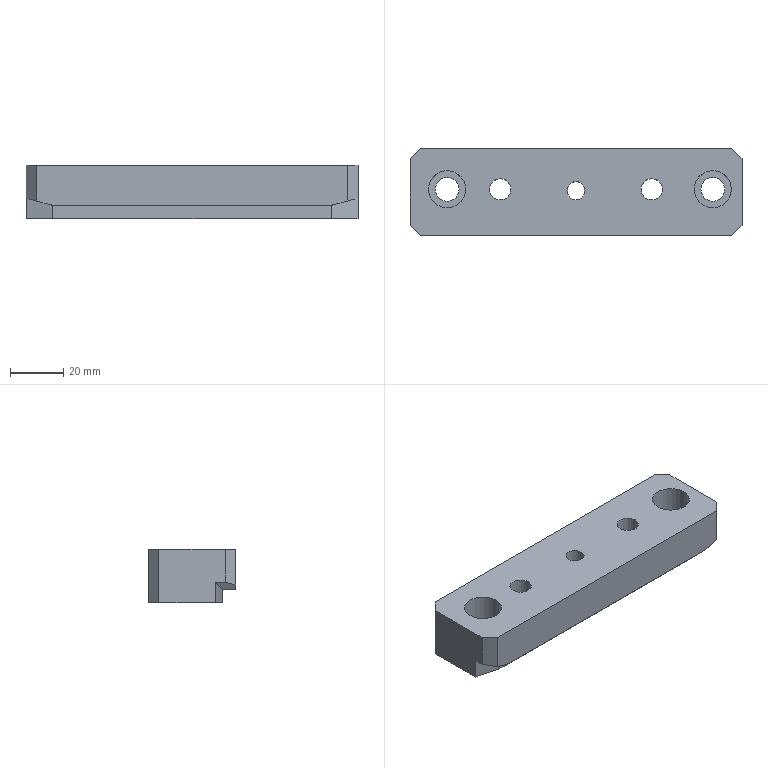Part | NX | features 20 2 | 1 solid | 25 faces | box 125 x 33 x 20 mm | volume 71448 mm3 | plane 18 | cylinder 7 | commonest cylinder face diameters 8.001 x2 9 x2 14 x2 6.8 x1
STEP:
#1=CARTESIAN_POINT('',(3433.002,435.,-3.5));
#2=VERTEX_POINT('',#1);
#3=CARTESIAN_POINT('',(3428.502,435.,-3.5));
#4=DIRECTION('',(0.,0.,-1.));
#5=DIRECTION('',(1.,0.,0.));
#6=AXIS2_PLACEMENT_3D('',#3,#4,#5);
#7=CIRCLE('',#6,4.5);
#8=EDGE_CURVE('',#2,#2,#7,.T.);
#9=ORIENTED_EDGE('',*,*,#8,.F.);
#10=EDGE_LOOP('',(#9));
#11=FACE_BOUND('',#10,.T.);
#12=CARTESIAN_POINT('',(3380.402,434.5,-3.5));
#13=VERTEX_POINT('',#12);
#14=CARTESIAN_POINT('',(3377.002,434.5,-3.5));
#15=DIRECTION('',(0.,0.,-1.));
#16=DIRECTION('',(1.,0.,0.));
#17=AXIS2_PLACEMENT_3D('',#14,#15,#16);
#18=CIRCLE('',#17,3.4);
#19=EDGE_CURVE('',#13,#13,#18,.T.);
#20=ORIENTED_EDGE('',*,*,#19,.F.);
#21=EDGE_LOOP('',(#20));
#22=FACE_BOUND('',#21,.T.);
#23=CARTESIAN_POINT('',(3333.002,435.,-3.5));
#24=VERTEX_POINT('',#23);
#25=CARTESIAN_POINT('',(3328.502,435.,-3.5));
#26=DIRECTION('',(0.,0.,1.));
#27=DIRECTION('',(1.,0.,0.));
#28=AXIS2_PLACEMENT_3D('',#25,#26,#27);
#29=CIRCLE('',#28,4.5);
#30=EDGE_CURVE('',#24,#24,#29,.T.);
#31=ORIENTED_EDGE('',*,*,#30,.T.);
#32=EDGE_LOOP('',(#31));
#33=FACE_BOUND('',#32,.T.);
#34=CARTESIAN_POINT('',(3429.501,422.5,-3.5));
#35=VERTEX_POINT('',#34);
#36=CARTESIAN_POINT('',(3324.501,422.5,-3.5));
#37=VERTEX_POINT('',#36);
#38=CARTESIAN_POINT('',(3410.501,422.5,-3.5));
#39=DIRECTION('',(-1.,0.,0.));
#40=VECTOR('',#39,1000.);
#41=LINE('',#38,#40);
#42=EDGE_CURVE('',#35,#37,#41,.T.);
#43=ORIENTED_EDGE('',*,*,#42,.T.);
#44=CARTESIAN_POINT('',(3314.502,425.179,-3.5));
#45=VERTEX_POINT('',#44);
#46=CARTESIAN_POINT('',(3324.501,422.5,-3.5));
#47=DIRECTION('',(-0.9659,0.2588,0.));
#48=VECTOR('',#47,1000.);
#49=LINE('',#46,#48);
#50=EDGE_CURVE('',#37,#45,#49,.T.);
#51=ORIENTED_EDGE('',*,*,#50,.T.);
#52=CARTESIAN_POINT('',(3314.502,446.5,-3.5));
#53=VERTEX_POINT('',#52);
#54=CARTESIAN_POINT('',(3314.502,417.5,-3.5));
#55=DIRECTION('',(0.,1.,0.));
#56=VECTOR('',#55,1000.);
#57=LINE('',#54,#56);
#58=EDGE_CURVE('',#45,#53,#57,.T.);
#59=ORIENTED_EDGE('',*,*,#58,.T.);
#60=CARTESIAN_POINT('',(3318.502,450.5,-3.5));
#61=VERTEX_POINT('',#60);
#62=CARTESIAN_POINT('',(3318.502,450.5,-3.5));
#63=DIRECTION('',(-0.7071,-0.7071,0.));
#64=VECTOR('',#63,1000.);
#65=LINE('',#62,#64);
#66=EDGE_CURVE('',#61,#53,#65,.T.);
#67=ORIENTED_EDGE('',*,*,#66,.F.);
#68=CARTESIAN_POINT('',(3435.502,450.5,-3.5));
#69=VERTEX_POINT('',#68);
#70=CARTESIAN_POINT('',(3432.502,450.5,-3.5));
#71=DIRECTION('',(1.,0.,0.));
#72=VECTOR('',#71,1000.);
#73=LINE('',#70,#72);
#74=EDGE_CURVE('',#61,#69,#73,.T.);
#75=ORIENTED_EDGE('',*,*,#74,.T.);
#76=CARTESIAN_POINT('',(3439.502,446.5,-3.5));
#77=VERTEX_POINT('',#76);
#78=CARTESIAN_POINT('',(3439.502,446.5,-3.5));
#79=DIRECTION('',(-0.7071,0.7071,0.));
#80=VECTOR('',#79,1000.);
#81=LINE('',#78,#80);
#82=EDGE_CURVE('',#77,#69,#81,.T.);
#83=ORIENTED_EDGE('',*,*,#82,.F.);
#84=CARTESIAN_POINT('',(3439.502,425.18,-3.5));
#85=VERTEX_POINT('',#84);
#86=CARTESIAN_POINT('',(3439.502,450.5,-3.5));
#87=DIRECTION('',(0.,-1.,0.));
#88=VECTOR('',#87,1000.);
#89=LINE('',#86,#88);
#90=EDGE_CURVE('',#77,#85,#89,.T.);
#91=ORIENTED_EDGE('',*,*,#90,.T.);
#92=CARTESIAN_POINT('',(3439.502,425.18,-3.5));
#93=DIRECTION('',(-0.9659,-0.2588,0.));
#94=VECTOR('',#93,1000.);
#95=LINE('',#92,#94);
#96=EDGE_CURVE('',#85,#35,#95,.T.);
#97=ORIENTED_EDGE('',*,*,#96,.T.);
#98=EDGE_LOOP('',(#43,#51,#59,#67,#75,#83,#91,#97));
#99=FACE_BOUND('',#98,.T.);
#100=CARTESIAN_POINT('',(3352.503,435.,-3.5));
#101=VERTEX_POINT('',#100);
#102=CARTESIAN_POINT('',(3348.502,435.,-3.5));
#103=DIRECTION('',(0.,0.,1.));
#104=DIRECTION('',(1.,0.,0.));
#105=AXIS2_PLACEMENT_3D('',#102,#103,#104);
#106=CIRCLE('',#105,4.);
#107=EDGE_CURVE('',#101,#101,#106,.T.);
#108=ORIENTED_EDGE('',*,*,#107,.T.);
#109=EDGE_LOOP('',(#108));
#110=FACE_BOUND('',#109,.T.);
#111=CARTESIAN_POINT('',(3409.503,435.,-3.5));
#112=VERTEX_POINT('',#111);
#113=CARTESIAN_POINT('',(3405.502,435.,-3.5));
#114=DIRECTION('',(0.,0.,-1.));
#115=DIRECTION('',(1.,0.,0.));
#116=AXIS2_PLACEMENT_3D('',#113,#114,#115);
#117=CIRCLE('',#116,4.);
#118=EDGE_CURVE('',#112,#112,#117,.T.);
#119=ORIENTED_EDGE('',*,*,#118,.F.);
#120=EDGE_LOOP('',(#119));
#121=FACE_BOUND('',#120,.T.);
#122=CARTESIAN_POINT('',(3502.502,450.5,-3.5));
#123=DIRECTION('',(0.,0.,1.));
#124=DIRECTION('',(-1.,0.,0.));
#125=AXIS2_PLACEMENT_3D('',#122,#123,#124);
#126=PLANE('',#125);
#127=ADVANCED_FACE('',(#11,#22,#33,#99,#110,#121),#126,.F.);
#128=CARTESIAN_POINT('',(3324.502,417.5,1.5));
#129=VERTEX_POINT('',#128);
#130=CARTESIAN_POINT('',(3429.502,417.5,1.5));
#131=VERTEX_POINT('',#130);
#132=CARTESIAN_POINT('',(3450.502,417.5,1.5));
#133=DIRECTION('',(1.,0.,0.));
#134=VECTOR('',#133,1000.);
#135=LINE('',#132,#134);
#136=EDGE_CURVE('',#129,#131,#135,.T.);
#137=ORIENTED_EDGE('',*,*,#136,.T.);
#138=CARTESIAN_POINT('',(3435.502,417.5,3.108));
#139=VERTEX_POINT('',#138);
#140=CARTESIAN_POINT('',(3429.502,417.5,1.5));
#141=DIRECTION('',(-0.9659,0.,-0.2588));
#142=VECTOR('',#141,1000.);
#143=LINE('',#140,#142);
#144=EDGE_CURVE('',#139,#131,#143,.T.);
#145=ORIENTED_EDGE('',*,*,#144,.F.);
#146=CARTESIAN_POINT('',(3435.502,417.5,16.5));
#147=VERTEX_POINT('',#146);
#148=CARTESIAN_POINT('',(3435.502,417.5,11.5));
#149=DIRECTION('',(0.,0.,-1.));
#150=VECTOR('',#149,1000.);
#151=LINE('',#148,#150);
#152=EDGE_CURVE('',#147,#139,#151,.T.);
#153=ORIENTED_EDGE('',*,*,#152,.F.);
#154=CARTESIAN_POINT('',(3318.502,417.5,16.5));
#155=VERTEX_POINT('',#154);
#156=CARTESIAN_POINT('',(3472.502,417.5,16.5));
#157=DIRECTION('',(-1.,0.,0.));
#158=VECTOR('',#157,1000.);
#159=LINE('',#156,#158);
#160=EDGE_CURVE('',#147,#155,#159,.T.);
#161=ORIENTED_EDGE('',*,*,#160,.T.);
#162=CARTESIAN_POINT('',(3318.502,417.5,3.108));
#163=VERTEX_POINT('',#162);
#164=CARTESIAN_POINT('',(3318.502,417.5,11.5));
#165=DIRECTION('',(0.,0.,1.));
#166=VECTOR('',#165,1000.);
#167=LINE('',#164,#166);
#168=EDGE_CURVE('',#163,#155,#167,.T.);
#169=ORIENTED_EDGE('',*,*,#168,.F.);
#170=CARTESIAN_POINT('',(3324.502,417.5,1.5));
#171=DIRECTION('',(-0.9659,0.,0.2588));
#172=VECTOR('',#171,1000.);
#173=LINE('',#170,#172);
#174=EDGE_CURVE('',#129,#163,#173,.T.);
#175=ORIENTED_EDGE('',*,*,#174,.F.);
#176=EDGE_LOOP('',(#137,#145,#153,#161,#169,#175));
#177=FACE_BOUND('',#176,.T.);
#178=CARTESIAN_POINT('',(3472.502,417.5,11.5));
#179=DIRECTION('',(0.,1.,0.));
#180=DIRECTION('',(0.,0.,1.));
#181=AXIS2_PLACEMENT_3D('',#178,#179,#180);
#182=PLANE('',#181);
#183=ADVANCED_FACE('',(#177),#182,.F.);
#184=CARTESIAN_POINT('',(3409.503,435.,16.5));
#185=VERTEX_POINT('',#184);
#186=CARTESIAN_POINT('',(3405.502,435.,16.5));
#187=DIRECTION('',(0.,0.,1.));
#188=DIRECTION('',(1.,0.,0.));
#189=AXIS2_PLACEMENT_3D('',#186,#187,#188);
#190=CIRCLE('',#189,4.);
#191=EDGE_CURVE('',#185,#185,#190,.T.);
#192=ORIENTED_EDGE('',*,*,#191,.F.);
#193=EDGE_LOOP('',(#192));
#194=FACE_BOUND('',#193,.T.);
#195=CARTESIAN_POINT('',(3352.503,435.,16.5));
#196=VERTEX_POINT('',#195);
#197=CARTESIAN_POINT('',(3348.502,435.,16.5));
#198=DIRECTION('',(0.,0.,1.));
#199=DIRECTION('',(1.,0.,0.));
#200=AXIS2_PLACEMENT_3D('',#197,#198,#199);
#201=CIRCLE('',#200,4.);
#202=EDGE_CURVE('',#196,#196,#201,.T.);
#203=ORIENTED_EDGE('',*,*,#202,.F.);
#204=EDGE_LOOP('',(#203));
#205=FACE_BOUND('',#204,.T.);
#206=CARTESIAN_POINT('',(3435.502,435.,16.5));
#207=VERTEX_POINT('',#206);
#208=CARTESIAN_POINT('',(3428.502,435.,16.5));
#209=DIRECTION('',(0.,0.,-1.));
#210=DIRECTION('',(1.,0.,0.));
#211=AXIS2_PLACEMENT_3D('',#208,#209,#210);
#212=CIRCLE('',#211,7.);
#213=EDGE_CURVE('',#207,#207,#212,.T.);
#214=ORIENTED_EDGE('',*,*,#213,.T.);
#215=EDGE_LOOP('',(#214));
#216=FACE_BOUND('',#215,.T.);
#217=CARTESIAN_POINT('',(3335.502,435.,16.5));
#218=VERTEX_POINT('',#217);
#219=CARTESIAN_POINT('',(3328.502,435.,16.5));
#220=DIRECTION('',(0.,0.,-1.));
#221=DIRECTION('',(1.,0.,0.));
#222=AXIS2_PLACEMENT_3D('',#219,#220,#221);
#223=CIRCLE('',#222,7.);
#224=EDGE_CURVE('',#218,#218,#223,.T.);
#225=ORIENTED_EDGE('',*,*,#224,.T.);
#226=EDGE_LOOP('',(#225));
#227=FACE_BOUND('',#226,.T.);
#228=ORIENTED_EDGE('',*,*,#160,.F.);
#229=CARTESIAN_POINT('',(3439.502,421.5,16.5));
#230=VERTEX_POINT('',#229);
#231=CARTESIAN_POINT('',(3435.502,417.5,16.5));
#232=DIRECTION('',(-0.7071,-0.7071,0.));
#233=VECTOR('',#232,1000.);
#234=LINE('',#231,#233);
#235=EDGE_CURVE('',#230,#147,#234,.T.);
#236=ORIENTED_EDGE('',*,*,#235,.F.);
#237=CARTESIAN_POINT('',(3439.502,446.5,16.5));
#238=VERTEX_POINT('',#237);
#239=CARTESIAN_POINT('',(3439.502,450.5,16.5));
#240=DIRECTION('',(0.,-1.,0.));
#241=VECTOR('',#240,1000.);
#242=LINE('',#239,#241);
#243=EDGE_CURVE('',#238,#230,#242,.T.);
#244=ORIENTED_EDGE('',*,*,#243,.F.);
#245=CARTESIAN_POINT('',(3435.502,450.5,16.5));
#246=VERTEX_POINT('',#245);
#247=CARTESIAN_POINT('',(3439.502,446.5,16.5));
#248=DIRECTION('',(0.7071,-0.7071,0.));
#249=VECTOR('',#248,1000.);
#250=LINE('',#247,#249);
#251=EDGE_CURVE('',#246,#238,#250,.T.);
#252=ORIENTED_EDGE('',*,*,#251,.F.);
#253=CARTESIAN_POINT('',(3318.502,450.5,16.5));
#254=VERTEX_POINT('',#253);
#255=CARTESIAN_POINT('',(3392.502,450.5,16.5));
#256=DIRECTION('',(1.,0.,0.));
#257=VECTOR('',#256,1000.);
#258=LINE('',#255,#257);
#259=EDGE_CURVE('',#254,#246,#258,.T.);
#260=ORIENTED_EDGE('',*,*,#259,.F.);
#261=CARTESIAN_POINT('',(3314.502,446.5,16.5));
#262=VERTEX_POINT('',#261);
#263=CARTESIAN_POINT('',(3318.502,450.5,16.5));
#264=DIRECTION('',(0.7071,0.7071,0.));
#265=VECTOR('',#264,1000.);
#266=LINE('',#263,#265);
#267=EDGE_CURVE('',#262,#254,#266,.T.);
#268=ORIENTED_EDGE('',*,*,#267,.F.);
#269=CARTESIAN_POINT('',(3314.502,421.5,16.5));
#270=VERTEX_POINT('',#269);
#271=CARTESIAN_POINT('',(3314.502,417.5,16.5));
#272=DIRECTION('',(0.,1.,0.));
#273=VECTOR('',#272,1000.);
#274=LINE('',#271,#273);
#275=EDGE_CURVE('',#270,#262,#274,.T.);
#276=ORIENTED_EDGE('',*,*,#275,.F.);
#277=CARTESIAN_POINT('',(3314.502,421.5,16.5));
#278=DIRECTION('',(-0.7071,0.7071,0.));
#279=VECTOR('',#278,1000.);
#280=LINE('',#277,#279);
#281=EDGE_CURVE('',#155,#270,#280,.T.);
#282=ORIENTED_EDGE('',*,*,#281,.F.);
#283=EDGE_LOOP('',(#228,#236,#244,#252,#260,#268,#276,#282));
#284=FACE_BOUND('',#283,.T.);
#285=CARTESIAN_POINT('',(3380.402,434.5,16.5));
#286=VERTEX_POINT('',#285);
#287=CARTESIAN_POINT('',(3377.002,434.5,16.5));
#288=DIRECTION('',(0.,0.,1.));
#289=DIRECTION('',(1.,0.,0.));
#290=AXIS2_PLACEMENT_3D('',#287,#288,#289);
#291=CIRCLE('',#290,3.4);
#292=EDGE_CURVE('',#286,#286,#291,.T.);
#293=ORIENTED_EDGE('',*,*,#292,.F.);
#294=EDGE_LOOP('',(#293));
#295=FACE_BOUND('',#294,.T.);
#296=CARTESIAN_POINT('',(3472.502,450.5,16.5));
#297=DIRECTION('',(0.,0.,1.));
#298=DIRECTION('',(-1.,0.,0.));
#299=AXIS2_PLACEMENT_3D('',#296,#297,#298);
#300=PLANE('',#299);
#301=ADVANCED_FACE('',(#194,#205,#216,#227,#284,#295),#300,.T.);
#302=CARTESIAN_POINT('',(3424.002,435.,6.5));
#303=VERTEX_POINT('',#302);
#304=CARTESIAN_POINT('',(3428.502,435.,6.5));
#305=DIRECTION('',(0.,0.,1.));
#306=DIRECTION('',(-1.,0.,0.));
#307=AXIS2_PLACEMENT_3D('',#304,#305,#306);
#308=CIRCLE('',#307,4.5);
#309=EDGE_CURVE('',#303,#303,#308,.T.);
#310=ORIENTED_EDGE('',*,*,#309,.F.);
#311=EDGE_LOOP('',(#310));
#312=FACE_BOUND('',#311,.T.);
#313=CARTESIAN_POINT('',(3421.502,435.,6.5));
#314=VERTEX_POINT('',#313);
#315=CARTESIAN_POINT('',(3428.502,435.,6.5));
#316=DIRECTION('',(0.,0.,-1.));
#317=DIRECTION('',(-1.,0.,0.));
#318=AXIS2_PLACEMENT_3D('',#315,#316,#317);
#319=CIRCLE('',#318,7.);
#320=EDGE_CURVE('',#314,#314,#319,.T.);
#321=ORIENTED_EDGE('',*,*,#320,.F.);
#322=EDGE_LOOP('',(#321));
#323=FACE_BOUND('',#322,.T.);
#324=CARTESIAN_POINT('',(3428.502,432.5,6.5));
#325=DIRECTION('',(0.,0.,-1.));
#326=DIRECTION('',(1.,0.,0.));
#327=AXIS2_PLACEMENT_3D('',#324,#325,#326);
#328=PLANE('',#327);
#329=ADVANCED_FACE('',(#312,#323),#328,.F.);
#330=CARTESIAN_POINT('',(3429.502,422.5,1.5));
#331=VERTEX_POINT('',#330);
#332=CARTESIAN_POINT('',(3429.502,425.18,1.5));
#333=DIRECTION('',(0.,1.,0.));
#334=VECTOR('',#333,1000.);
#335=LINE('',#332,#334);
#336=EDGE_CURVE('',#131,#331,#335,.T.);
#337=ORIENTED_EDGE('',*,*,#336,.T.);
#338=CARTESIAN_POINT('',(3439.502,425.18,4.179));
#339=VERTEX_POINT('',#338);
#340=CARTESIAN_POINT('',(3438.875,425.012,4.011));
#341=DIRECTION('',(0.9351,0.2506,0.2506));
#342=VECTOR('',#341,1000.);
#343=LINE('',#340,#342);
#344=EDGE_CURVE('',#331,#339,#343,.T.);
#345=ORIENTED_EDGE('',*,*,#344,.T.);
#346=CARTESIAN_POINT('',(3439.502,421.5,4.179));
#347=VERTEX_POINT('',#346);
#348=CARTESIAN_POINT('',(3439.502,417.5,4.179));
#349=DIRECTION('',(0.,-1.,0.));
#350=VECTOR('',#349,1000.);
#351=LINE('',#348,#350);
#352=EDGE_CURVE('',#339,#347,#351,.T.);
#353=ORIENTED_EDGE('',*,*,#352,.T.);
#354=CARTESIAN_POINT('',(3422.451,404.449,-0.3894));
#355=DIRECTION('',(0.6947,0.6947,0.1862));
#356=VECTOR('',#355,1000.);
#357=LINE('',#354,#356);
#358=EDGE_CURVE('',#139,#347,#357,.T.);
#359=ORIENTED_EDGE('',*,*,#358,.F.);
#360=ORIENTED_EDGE('',*,*,#144,.T.);
#361=EDGE_LOOP('',(#337,#345,#353,#359,#360));
#362=FACE_BOUND('',#361,.T.);
#363=CARTESIAN_POINT('',(3429.502,396.891,1.5));
#364=DIRECTION('',(0.2588,0.,-0.9659));
#365=DIRECTION('',(0.9659,0.,0.2588));
#366=AXIS2_PLACEMENT_3D('',#363,#364,#365);
#367=PLANE('',#366);
#368=ADVANCED_FACE('',(#362),#367,.T.);
#369=CARTESIAN_POINT('',(3324.002,435.,6.5));
#370=VERTEX_POINT('',#369);
#371=CARTESIAN_POINT('',(3328.502,435.,6.5));
#372=DIRECTION('',(0.,0.,1.));
#373=DIRECTION('',(-1.,0.,0.));
#374=AXIS2_PLACEMENT_3D('',#371,#372,#373);
#375=CIRCLE('',#374,4.5);
#376=EDGE_CURVE('',#370,#370,#375,.T.);
#377=ORIENTED_EDGE('',*,*,#376,.F.);
#378=EDGE_LOOP('',(#377));
#379=FACE_BOUND('',#378,.T.);
#380=CARTESIAN_POINT('',(3321.502,435.,6.5));
#381=VERTEX_POINT('',#380);
#382=CARTESIAN_POINT('',(3328.502,435.,6.5));
#383=DIRECTION('',(0.,0.,-1.));
#384=DIRECTION('',(-1.,0.,0.));
#385=AXIS2_PLACEMENT_3D('',#382,#383,#384);
#386=CIRCLE('',#385,7.);
#387=EDGE_CURVE('',#381,#381,#386,.T.);
#388=ORIENTED_EDGE('',*,*,#387,.F.);
#389=EDGE_LOOP('',(#388));
#390=FACE_BOUND('',#389,.T.);
#391=CARTESIAN_POINT('',(3328.502,432.5,6.5));
#392=DIRECTION('',(0.,0.,-1.));
#393=DIRECTION('',(-1.,0.,0.));
#394=AXIS2_PLACEMENT_3D('',#391,#392,#393);
#395=PLANE('',#394);
#396=ADVANCED_FACE('',(#379,#390),#395,.F.);
#397=ORIENTED_EDGE('',*,*,#213,.F.);
#398=EDGE_LOOP('',(#397));
#399=FACE_BOUND('',#398,.T.);
#400=ORIENTED_EDGE('',*,*,#320,.T.);
#401=EDGE_LOOP('',(#400));
#402=FACE_BOUND('',#401,.T.);
#403=CARTESIAN_POINT('',(3428.502,435.,42.5));
#404=DIRECTION('',(0.,0.,-1.));
#405=DIRECTION('',(1.,0.,0.));
#406=AXIS2_PLACEMENT_3D('',#403,#404,#405);
#407=CYLINDRICAL_SURFACE('',#406,7.);
#408=ADVANCED_FACE('',(#399,#402),#407,.F.);
#409=ORIENTED_EDGE('',*,*,#235,.T.);
#410=ORIENTED_EDGE('',*,*,#152,.T.);
#411=ORIENTED_EDGE('',*,*,#358,.T.);
#412=CARTESIAN_POINT('',(3439.502,421.5,11.5));
#413=DIRECTION('',(0.,0.,1.));
#414=VECTOR('',#413,1000.);
#415=LINE('',#412,#414);
#416=EDGE_CURVE('',#347,#230,#415,.T.);
#417=ORIENTED_EDGE('',*,*,#416,.T.);
#418=EDGE_LOOP('',(#409,#410,#411,#417));
#419=FACE_BOUND('',#418,.T.);
#420=CARTESIAN_POINT('',(3435.502,417.5,11.5));
#421=DIRECTION('',(-0.7071,0.7071,0.));
#422=DIRECTION('',(0.,0.,-1.));
#423=AXIS2_PLACEMENT_3D('',#420,#421,#422);
#424=PLANE('',#423);
#425=ADVANCED_FACE('',(#419),#424,.F.);
#426=ORIENTED_EDGE('',*,*,#387,.T.);
#427=EDGE_LOOP('',(#426));
#428=FACE_BOUND('',#427,.T.);
#429=ORIENTED_EDGE('',*,*,#224,.F.);
#430=EDGE_LOOP('',(#429));
#431=FACE_BOUND('',#430,.T.);
#432=CARTESIAN_POINT('',(3328.502,435.,42.5));
#433=DIRECTION('',(0.,0.,-1.));
#434=DIRECTION('',(-1.,0.,0.));
#435=AXIS2_PLACEMENT_3D('',#432,#433,#434);
#436=CYLINDRICAL_SURFACE('',#435,7.);
#437=ADVANCED_FACE('',(#428,#431),#436,.F.);
#438=ORIENTED_EDGE('',*,*,#352,.F.);
#439=CARTESIAN_POINT('',(3439.502,425.18,3.5));
#440=DIRECTION('',(0.,0.,-1.));
#441=VECTOR('',#440,1000.);
#442=LINE('',#439,#441);
#443=EDGE_CURVE('',#339,#85,#442,.T.);
#444=ORIENTED_EDGE('',*,*,#443,.T.);
#445=ORIENTED_EDGE('',*,*,#90,.F.);
#446=CARTESIAN_POINT('',(3439.502,446.5,11.5));
#447=DIRECTION('',(0.,0.,-1.));
#448=VECTOR('',#447,1000.);
#449=LINE('',#446,#448);
#450=EDGE_CURVE('',#238,#77,#449,.T.);
#451=ORIENTED_EDGE('',*,*,#450,.F.);
#452=ORIENTED_EDGE('',*,*,#243,.T.);
#453=ORIENTED_EDGE('',*,*,#416,.F.);
#454=EDGE_LOOP('',(#438,#444,#445,#451,#452,#453));
#455=FACE_BOUND('',#454,.T.);
#456=CARTESIAN_POINT('',(3439.502,450.5,11.5));
#457=DIRECTION('',(-1.,0.,0.));
#458=DIRECTION('',(0.,0.,-1.));
#459=AXIS2_PLACEMENT_3D('',#456,#457,#458);
#460=PLANE('',#459);
#461=ADVANCED_FACE('',(#455),#460,.F.);
#462=CARTESIAN_POINT('',(3429.501,422.5,1.5));
#463=VERTEX_POINT('',#462);
#464=CARTESIAN_POINT('',(3439.502,425.18,1.5));
#465=DIRECTION('',(0.9659,0.2588,0.));
#466=VECTOR('',#465,1000.);
#467=LINE('',#464,#466);
#468=EDGE_CURVE('',#463,#331,#467,.T.);
#469=ORIENTED_EDGE('',*,*,#468,.F.);
#470=CARTESIAN_POINT('',(3429.501,422.5,3.5));
#471=DIRECTION('',(0.,0.,1.));
#472=VECTOR('',#471,1000.);
#473=LINE('',#470,#472);
#474=EDGE_CURVE('',#35,#463,#473,.T.);
#475=ORIENTED_EDGE('',*,*,#474,.F.);
#476=ORIENTED_EDGE('',*,*,#96,.F.);
#477=ORIENTED_EDGE('',*,*,#443,.F.);
#478=ORIENTED_EDGE('',*,*,#344,.F.);
#479=EDGE_LOOP('',(#469,#475,#476,#477,#478));
#480=FACE_BOUND('',#479,.T.);
#481=CARTESIAN_POINT('',(3439.502,425.18,3.5));
#482=DIRECTION('',(-0.2588,0.9659,0.));
#483=DIRECTION('',(0.9659,0.2588,0.));
#484=AXIS2_PLACEMENT_3D('',#481,#482,#483);
#485=PLANE('',#484);
#486=ADVANCED_FACE('',(#480),#485,.F.);
#487=ORIENTED_EDGE('',*,*,#309,.T.);
#488=EDGE_LOOP('',(#487));
#489=FACE_BOUND('',#488,.T.);
#490=ORIENTED_EDGE('',*,*,#8,.T.);
#491=EDGE_LOOP('',(#490));
#492=FACE_BOUND('',#491,.T.);
#493=CARTESIAN_POINT('',(3428.502,435.,42.5));
#494=DIRECTION('',(0.,0.,-1.));
#495=DIRECTION('',(1.,0.,0.));
#496=AXIS2_PLACEMENT_3D('',#493,#494,#495);
#497=CYLINDRICAL_SURFACE('',#496,4.5);
#498=ADVANCED_FACE('',(#489,#492),#497,.F.);
#499=CARTESIAN_POINT('',(3314.502,421.5,4.179));
#500=VERTEX_POINT('',#499);
#501=CARTESIAN_POINT('',(3314.502,421.5,11.5));
#502=DIRECTION('',(0.,0.,-1.));
#503=VECTOR('',#502,1000.);
#504=LINE('',#501,#503);
#505=EDGE_CURVE('',#270,#500,#504,.T.);
#506=ORIENTED_EDGE('',*,*,#505,.T.);
#507=CARTESIAN_POINT('',(3331.554,404.449,-0.3894));
#508=DIRECTION('',(0.6947,-0.6947,-0.1862));
#509=VECTOR('',#508,1000.);
#510=LINE('',#507,#509);
#511=EDGE_CURVE('',#500,#163,#510,.T.);
#512=ORIENTED_EDGE('',*,*,#511,.T.);
#513=ORIENTED_EDGE('',*,*,#168,.T.);
#514=ORIENTED_EDGE('',*,*,#281,.T.);
#515=EDGE_LOOP('',(#506,#512,#513,#514));
#516=FACE_BOUND('',#515,.T.);
#517=CARTESIAN_POINT('',(3314.502,421.5,11.5));
#518=DIRECTION('',(0.7071,0.7071,0.));
#519=DIRECTION('',(0.,0.,-1.));
#520=AXIS2_PLACEMENT_3D('',#517,#518,#519);
#521=PLANE('',#520);
#522=ADVANCED_FACE('',(#516),#521,.F.);
#523=ORIENTED_EDGE('',*,*,#30,.F.);
#524=EDGE_LOOP('',(#523));
#525=FACE_BOUND('',#524,.T.);
#526=ORIENTED_EDGE('',*,*,#376,.T.);
#527=EDGE_LOOP('',(#526));
#528=FACE_BOUND('',#527,.T.);
#529=CARTESIAN_POINT('',(3328.502,435.,42.5));
#530=DIRECTION('',(0.,0.,-1.));
#531=DIRECTION('',(-1.,0.,0.));
#532=AXIS2_PLACEMENT_3D('',#529,#530,#531);
#533=CYLINDRICAL_SURFACE('',#532,4.5);
#534=ADVANCED_FACE('',(#525,#528),#533,.F.);
#535=ORIENTED_EDGE('',*,*,#58,.F.);
#536=CARTESIAN_POINT('',(3314.502,425.179,4.179));
#537=VERTEX_POINT('',#536);
#538=CARTESIAN_POINT('',(3314.502,425.179,3.5));
#539=DIRECTION('',(0.,0.,-1.));
#540=VECTOR('',#539,1000.);
#541=LINE('',#538,#540);
#542=EDGE_CURVE('',#537,#45,#541,.T.);
#543=ORIENTED_EDGE('',*,*,#542,.F.);
#544=CARTESIAN_POINT('',(3314.502,425.179,4.179));
#545=DIRECTION('',(0.,1.,0.));
#546=VECTOR('',#545,1000.);
#547=LINE('',#544,#546);
#548=EDGE_CURVE('',#500,#537,#547,.T.);
#549=ORIENTED_EDGE('',*,*,#548,.F.);
#550=ORIENTED_EDGE('',*,*,#505,.F.);
#551=ORIENTED_EDGE('',*,*,#275,.T.);
#552=CARTESIAN_POINT('',(3314.502,446.5,11.5));
#553=DIRECTION('',(0.,0.,1.));
#554=VECTOR('',#553,1000.);
#555=LINE('',#552,#554);
#556=EDGE_CURVE('',#53,#262,#555,.T.);
#557=ORIENTED_EDGE('',*,*,#556,.F.);
#558=EDGE_LOOP('',(#535,#543,#549,#550,#551,#557));
#559=FACE_BOUND('',#558,.T.);
#560=CARTESIAN_POINT('',(3314.502,417.5,11.5));
#561=DIRECTION('',(1.,0.,0.));
#562=DIRECTION('',(0.,0.,1.));
#563=AXIS2_PLACEMENT_3D('',#560,#561,#562);
#564=PLANE('',#563);
#565=ADVANCED_FACE('',(#559),#564,.F.);
#566=ORIENTED_EDGE('',*,*,#548,.T.);
#567=CARTESIAN_POINT('',(3324.501,422.5,1.5));
#568=VERTEX_POINT('',#567);
#569=CARTESIAN_POINT('',(3324.501,422.5,1.5));
#570=DIRECTION('',(0.9351,-0.2506,-0.2506));
#571=VECTOR('',#570,1000.);
#572=LINE('',#569,#571);
#573=EDGE_CURVE('',#537,#568,#572,.T.);
#574=ORIENTED_EDGE('',*,*,#573,.T.);
#575=CARTESIAN_POINT('',(3324.502,422.5,1.5));
#576=VERTEX_POINT('',#575);
#577=CARTESIAN_POINT('',(3324.502,422.5,1.5));
#578=DIRECTION('',(0.9659,0.,-0.2588));
#579=VECTOR('',#578,1000.);
#580=LINE('',#577,#579);
#581=EDGE_CURVE('',#568,#576,#580,.T.);
#582=ORIENTED_EDGE('',*,*,#581,.T.);
#583=CARTESIAN_POINT('',(3324.502,417.5,1.5));
#584=DIRECTION('',(0.,-1.,0.));
#585=VECTOR('',#584,1000.);
#586=LINE('',#583,#585);
#587=EDGE_CURVE('',#576,#129,#586,.T.);
#588=ORIENTED_EDGE('',*,*,#587,.T.);
#589=ORIENTED_EDGE('',*,*,#174,.T.);
#590=ORIENTED_EDGE('',*,*,#511,.F.);
#591=EDGE_LOOP('',(#566,#574,#582,#588,#589,#590));
#592=FACE_BOUND('',#591,.T.);
#593=CARTESIAN_POINT('',(3324.502,396.891,1.5));
#594=DIRECTION('',(-0.2588,0.,-0.9659));
#595=DIRECTION('',(0.9659,0.,-0.2588));
#596=AXIS2_PLACEMENT_3D('',#593,#594,#595);
#597=PLANE('',#596);
#598=ADVANCED_FACE('',(#592),#597,.T.);
#599=ORIENTED_EDGE('',*,*,#50,.F.);
#600=CARTESIAN_POINT('',(3324.501,422.5,3.5));
#601=DIRECTION('',(0.,0.,1.));
#602=VECTOR('',#601,1000.);
#603=LINE('',#600,#602);
#604=EDGE_CURVE('',#37,#568,#603,.T.);
#605=ORIENTED_EDGE('',*,*,#604,.T.);
#606=ORIENTED_EDGE('',*,*,#573,.F.);
#607=ORIENTED_EDGE('',*,*,#542,.T.);
#608=EDGE_LOOP('',(#599,#605,#606,#607));
#609=FACE_BOUND('',#608,.T.);
#610=CARTESIAN_POINT('',(3324.501,422.5,3.5));
#611=DIRECTION('',(0.2588,0.9659,0.));
#612=DIRECTION('',(0.9659,-0.2588,0.));
#613=AXIS2_PLACEMENT_3D('',#610,#611,#612);
#614=PLANE('',#613);
#615=ADVANCED_FACE('',(#609),#614,.F.);
#616=ORIENTED_EDGE('',*,*,#66,.T.);
#617=ORIENTED_EDGE('',*,*,#556,.T.);
#618=ORIENTED_EDGE('',*,*,#267,.T.);
#619=CARTESIAN_POINT('',(3318.502,450.5,11.5));
#620=DIRECTION('',(0.,0.,-1.));
#621=VECTOR('',#620,1000.);
#622=LINE('',#619,#621);
#623=EDGE_CURVE('',#254,#61,#622,.T.);
#624=ORIENTED_EDGE('',*,*,#623,.T.);
#625=EDGE_LOOP('',(#616,#617,#618,#624));
#626=FACE_BOUND('',#625,.T.);
#627=CARTESIAN_POINT('',(3318.502,450.5,11.5));
#628=DIRECTION('',(0.7071,-0.7071,0.));
#629=DIRECTION('',(0.,0.,-1.));
#630=AXIS2_PLACEMENT_3D('',#627,#628,#629);
#631=PLANE('',#630);
#632=ADVANCED_FACE('',(#626),#631,.F.);
#633=ORIENTED_EDGE('',*,*,#82,.T.);
#634=CARTESIAN_POINT('',(3435.502,450.5,11.5));
#635=DIRECTION('',(0.,0.,1.));
#636=VECTOR('',#635,1000.);
#637=LINE('',#634,#636);
#638=EDGE_CURVE('',#69,#246,#637,.T.);
#639=ORIENTED_EDGE('',*,*,#638,.T.);
#640=ORIENTED_EDGE('',*,*,#251,.T.);
#641=ORIENTED_EDGE('',*,*,#450,.T.);
#642=EDGE_LOOP('',(#633,#639,#640,#641));
#643=FACE_BOUND('',#642,.T.);
#644=CARTESIAN_POINT('',(3439.502,446.5,11.5));
#645=DIRECTION('',(-0.7071,-0.7071,0.));
#646=DIRECTION('',(0.,0.,-1.));
#647=AXIS2_PLACEMENT_3D('',#644,#645,#646);
#648=PLANE('',#647);
#649=ADVANCED_FACE('',(#643),#648,.F.);
#650=ORIENTED_EDGE('',*,*,#638,.F.);
#651=ORIENTED_EDGE('',*,*,#74,.F.);
#652=ORIENTED_EDGE('',*,*,#623,.F.);
#653=ORIENTED_EDGE('',*,*,#259,.T.);
#654=EDGE_LOOP('',(#650,#651,#652,#653));
#655=FACE_BOUND('',#654,.T.);
#656=CARTESIAN_POINT('',(3392.502,450.5,11.5));
#657=DIRECTION('',(0.,-1.,0.));
#658=DIRECTION('',(0.,0.,-1.));
#659=AXIS2_PLACEMENT_3D('',#656,#657,#658);
#660=PLANE('',#659);
#661=ADVANCED_FACE('',(#655),#660,.F.);
#662=CARTESIAN_POINT('',(3440.501,422.5,1.5));
#663=DIRECTION('',(1.,0.,0.));
#664=VECTOR('',#663,1000.);
#665=LINE('',#662,#664);
#666=EDGE_CURVE('',#576,#463,#665,.T.);
#667=ORIENTED_EDGE('',*,*,#666,.T.);
#668=ORIENTED_EDGE('',*,*,#468,.T.);
#669=ORIENTED_EDGE('',*,*,#336,.F.);
#670=ORIENTED_EDGE('',*,*,#136,.F.);
#671=ORIENTED_EDGE('',*,*,#587,.F.);
#672=EDGE_LOOP('',(#667,#668,#669,#670,#671));
#673=FACE_BOUND('',#672,.T.);
#674=CARTESIAN_POINT('',(3472.773,396.891,1.5));
#675=DIRECTION('',(0.,0.,-1.));
#676=DIRECTION('',(1.,0.,0.));
#677=AXIS2_PLACEMENT_3D('',#674,#675,#676);
#678=PLANE('',#677);
#679=ADVANCED_FACE('',(#673),#678,.T.);
#680=ORIENTED_EDGE('',*,*,#474,.T.);
#681=ORIENTED_EDGE('',*,*,#666,.F.);
#682=ORIENTED_EDGE('',*,*,#581,.F.);
#683=ORIENTED_EDGE('',*,*,#604,.F.);
#684=ORIENTED_EDGE('',*,*,#42,.F.);
#685=EDGE_LOOP('',(#680,#681,#682,#683,#684));
#686=FACE_BOUND('',#685,.T.);
#687=CARTESIAN_POINT('',(3410.501,422.5,3.5));
#688=DIRECTION('',(0.,1.,0.));
#689=DIRECTION('',(0.,0.,1.));
#690=AXIS2_PLACEMENT_3D('',#687,#688,#689);
#691=PLANE('',#690);
#692=ADVANCED_FACE('',(#686),#691,.F.);
#693=ORIENTED_EDGE('',*,*,#292,.T.);
#694=EDGE_LOOP('',(#693));
#695=FACE_BOUND('',#694,.T.);
#696=ORIENTED_EDGE('',*,*,#19,.T.);
#697=EDGE_LOOP('',(#696));
#698=FACE_BOUND('',#697,.T.);
#699=CARTESIAN_POINT('',(3377.002,434.5,16.5));
#700=DIRECTION('',(0.,0.,-1.));
#701=DIRECTION('',(-1.,0.,0.));
#702=AXIS2_PLACEMENT_3D('',#699,#700,#701);
#703=CYLINDRICAL_SURFACE('',#702,3.4);
#704=ADVANCED_FACE('',(#695,#698),#703,.F.);
#705=ORIENTED_EDGE('',*,*,#202,.T.);
#706=EDGE_LOOP('',(#705));
#707=FACE_BOUND('',#706,.T.);
#708=ORIENTED_EDGE('',*,*,#107,.F.);
#709=EDGE_LOOP('',(#708));
#710=FACE_BOUND('',#709,.T.);
#711=CARTESIAN_POINT('',(3348.502,435.,-3.5));
#712=DIRECTION('',(0.,0.,1.));
#713=DIRECTION('',(-1.,0.,0.));
#714=AXIS2_PLACEMENT_3D('',#711,#712,#713);
#715=CYLINDRICAL_SURFACE('',#714,4.);
#716=ADVANCED_FACE('',(#707,#710),#715,.F.);
#717=ORIENTED_EDGE('',*,*,#191,.T.);
#718=EDGE_LOOP('',(#717));
#719=FACE_BOUND('',#718,.T.);
#720=ORIENTED_EDGE('',*,*,#118,.T.);
#721=EDGE_LOOP('',(#720));
#722=FACE_BOUND('',#721,.T.);
#723=CARTESIAN_POINT('',(3405.502,435.,-3.5));
#724=DIRECTION('',(0.,0.,1.));
#725=DIRECTION('',(1.,0.,0.));
#726=AXIS2_PLACEMENT_3D('',#723,#724,#725);
#727=CYLINDRICAL_SURFACE('',#726,4.);
#728=ADVANCED_FACE('',(#719,#722),#727,.F.);
#729=CLOSED_SHELL('',(#127,#183,#301,#329,#368,#396,#408,#425,#437,#461,#486,#498,#522,#534,#565,#598,#615,#632,#649,#661,#679,#692,#704,#716,#728));
#730=MANIFOLD_SOLID_BREP('',#729);
#731=(LENGTH_UNIT()NAMED_UNIT(*)SI_UNIT(.MILLI.,.METRE.));
#732=UNCERTAINTY_MEASURE_WITH_UNIT(LENGTH_MEASURE(0.00001),#731,'','');
#733=(NAMED_UNIT(*)PLANE_ANGLE_UNIT()SI_UNIT($,.RADIAN.));
#734=(NAMED_UNIT(*)SI_UNIT($,.STERADIAN.)SOLID_ANGLE_UNIT());
#735=(GEOMETRIC_REPRESENTATION_CONTEXT(3)GLOBAL_UNCERTAINTY_ASSIGNED_CONTEXT((#732))GLOBAL_UNIT_ASSIGNED_CONTEXT((#731,#733,#734))REPRESENTATION_CONTEXT('',''));
#736=ADVANCED_BREP_SHAPE_REPRESENTATION('',(#730),#735);